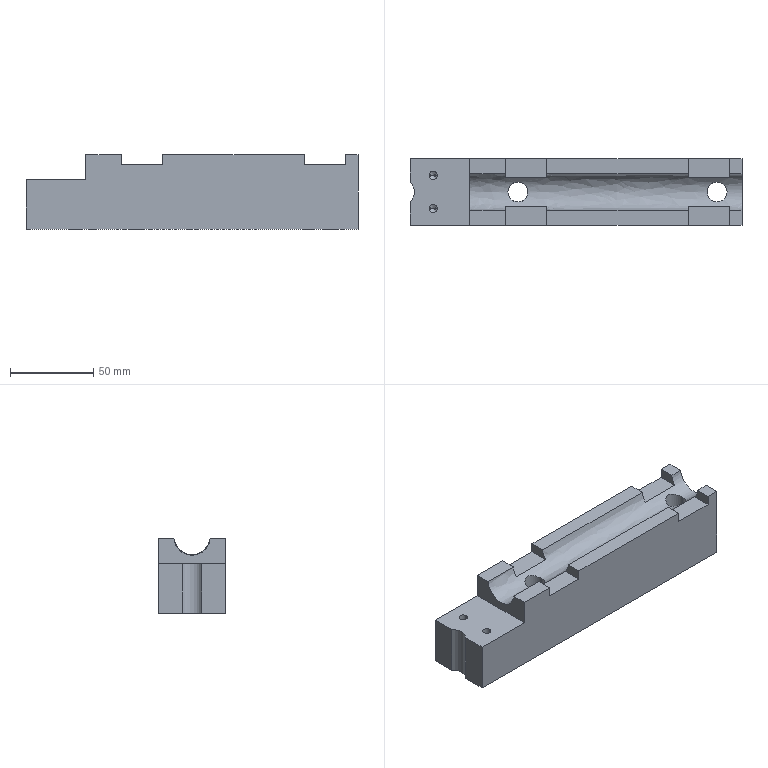NC program | NX | posted with a generic post
Lines 1 to 50 of 104568:
N10 G17 G21 G94 G90
(FLOOR_WALL , TOOL : D63)
N12 T01 M6
N14 G54
N16 G17 G0 G90 X-134.5 Y0. S6500 M3
N18 G43 Z30. H1
N20 Z7.
N22 G94 G1 Z4. F1250.
N24 X-131.5
N26 X131.5
N28 X134.5
N30 Z7.
N32 G0 Z30.
N34 X-134.5
N36 Z6.
N38 G1 Z3.
N40 X-131.5
N42 X131.5
N44 X134.5
N46 Z6.
N48 G0 Z30.
N50 X-134.5
N52 Z5.
N54 G1 Z2.
N56 X-131.5
N58 X131.5
N60 X134.5
N62 Z5.
N64 G0 Z30.
N66 X-134.5
N68 Z4.
N70 G1 Z1.
N72 X-131.5
N74 X131.5
N76 X134.5
N78 Z4.
N80 G0 Z30.
N82 X-134.5
N84 Z3.
N86 G1 Z0.
N88 X-131.5
N90 X131.5
N92 X134.5
N94 Z3.
N96 G0 Z30.
N98 M5